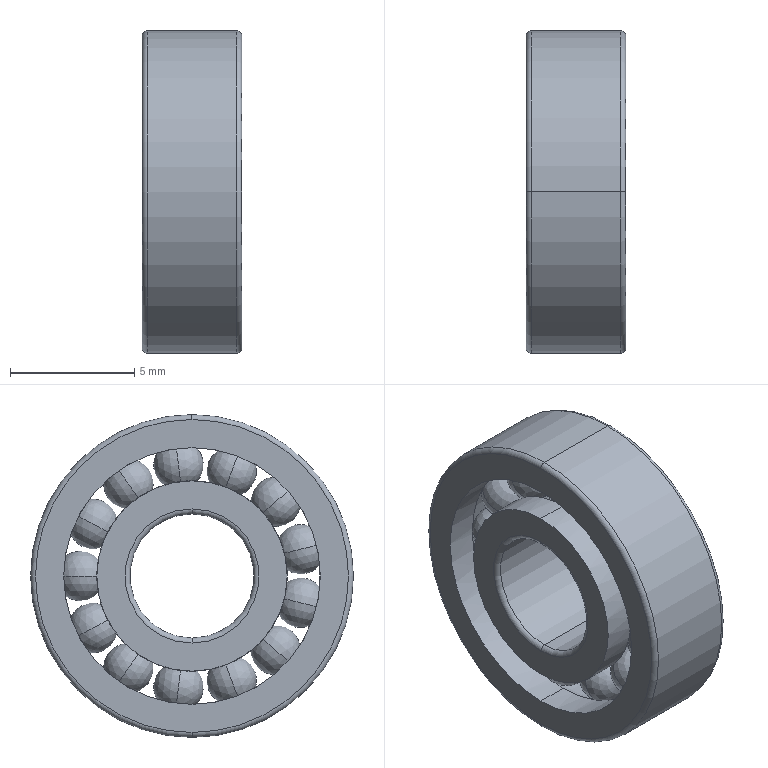Part | STEP file | deep groove ball bearings gb_Rolling bearings 619-5 GB 276-94 | 1 solid | 92 faces | box 4 x 13 x 13 mm | volume 336.475 mm3 | torus 50 | sphere 26 | cylinder 12 | plane 4 | commonest cylinder face diameters 7.667 x4 10.333 x4 5 x2 13 x2